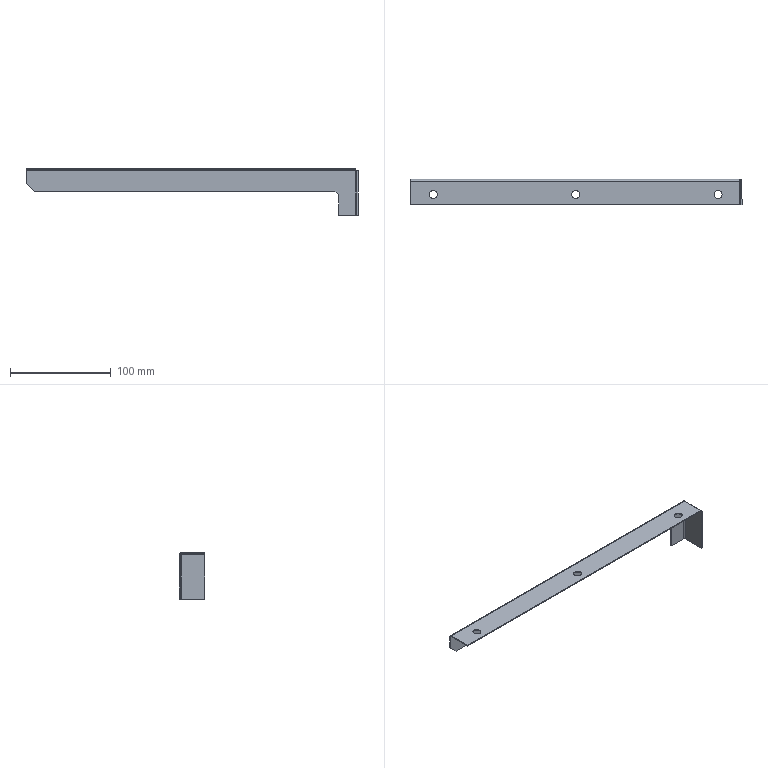Part | SolidWorks | features ICE 4, EdgeFlange 2, Chamfer 1, Fillet 1, FlatPattern 1, SMBaseFlange 1, SheetMetal 1 | 1 solid | 32 faces | box 330 x 25 x 46.5 mm | volume 16555 mm3 | plane 21 | cylinder 11 | commonest cylinder face diameters 8 x6 2 x2 4 x2 10 x1
STEP:
#1=CARTESIAN_POINT('',(-159.3,-14.,46.5));
#2=VERTEX_POINT('',#1);
#3=CARTESIAN_POINT('',(-167.3,-14.,46.5));
#4=VERTEX_POINT('',#3);
#5=CARTESIAN_POINT('',(-163.3,-14.,46.5));
#6=DIRECTION('',(0.,0.,-1.));
#7=DIRECTION('',(-1.,0.,0.));
#8=AXIS2_PLACEMENT_3D('',#5,#6,#7);
#9=CIRCLE('',#8,4.);
#10=EDGE_CURVE('',#2,#4,#9,.T.);
#11=ORIENTED_EDGE('',*,*,#10,.F.);
#12=CARTESIAN_POINT('',(-159.3,-14.,45.5));
#13=VERTEX_POINT('',#12);
#14=CARTESIAN_POINT('',(-159.3,-14.,46.5));
#15=DIRECTION('',(0.,0.,-1.));
#16=VECTOR('',#15,1000.);
#17=LINE('',#14,#16);
#18=EDGE_CURVE('',#2,#13,#17,.T.);
#19=ORIENTED_EDGE('',*,*,#18,.T.);
#20=CARTESIAN_POINT('',(-167.3,-14.,45.5));
#21=VERTEX_POINT('',#20);
#22=CARTESIAN_POINT('',(-163.3,-14.,45.5));
#23=DIRECTION('',(0.,0.,-1.));
#24=DIRECTION('',(-1.,0.,0.));
#25=AXIS2_PLACEMENT_3D('',#22,#23,#24);
#26=CIRCLE('',#25,4.);
#27=EDGE_CURVE('',#13,#21,#26,.T.);
#28=ORIENTED_EDGE('',*,*,#27,.T.);
#29=CARTESIAN_POINT('',(-167.3,-14.,46.5));
#30=DIRECTION('',(0.,0.,-1.));
#31=VECTOR('',#30,1000.);
#32=LINE('',#29,#31);
#33=EDGE_CURVE('',#4,#21,#32,.T.);
#34=ORIENTED_EDGE('',*,*,#33,.F.);
#35=EDGE_LOOP('',(#11,#19,#28,#34));
#36=FACE_OUTER_BOUND('',#35,.T.);
#37=CARTESIAN_POINT('',(-163.3,-14.,46.5));
#38=DIRECTION('',(0.,0.,-1.));
#39=DIRECTION('',(-1.,0.,0.));
#40=AXIS2_PLACEMENT_3D('',#37,#38,#39);
#41=CYLINDRICAL_SURFACE('',#40,4.);
#42=ADVANCED_FACE('',(#36),#41,.F.);
#43=CARTESIAN_POINT('',(-300.8,-14.,45.5));
#44=VERTEX_POINT('',#43);
#45=CARTESIAN_POINT('',(-308.8,-14.,45.5));
#46=VERTEX_POINT('',#45);
#47=CARTESIAN_POINT('',(-304.8,-14.,45.5));
#48=DIRECTION('',(0.,0.,-1.));
#49=DIRECTION('',(0.,-1.,0.));
#50=AXIS2_PLACEMENT_3D('',#47,#48,#49);
#51=CIRCLE('',#50,4.);
#52=EDGE_CURVE('',#44,#46,#51,.T.);
#53=ORIENTED_EDGE('',*,*,#52,.T.);
#54=CARTESIAN_POINT('',(-308.8,-14.,46.5));
#55=VERTEX_POINT('',#54);
#56=CARTESIAN_POINT('',(-308.8,-14.,-0.001));
#57=DIRECTION('',(0.,0.,1.));
#58=VECTOR('',#57,1000.);
#59=LINE('',#56,#58);
#60=EDGE_CURVE('',#46,#55,#59,.T.);
#61=ORIENTED_EDGE('',*,*,#60,.T.);
#62=CARTESIAN_POINT('',(-300.8,-14.,46.5));
#63=VERTEX_POINT('',#62);
#64=CARTESIAN_POINT('',(-304.8,-14.,46.5));
#65=DIRECTION('',(0.,0.,1.));
#66=DIRECTION('',(1.,0.,0.));
#67=AXIS2_PLACEMENT_3D('',#64,#65,#66);
#68=CIRCLE('',#67,4.);
#69=EDGE_CURVE('',#55,#63,#68,.T.);
#70=ORIENTED_EDGE('',*,*,#69,.T.);
#71=CARTESIAN_POINT('',(-300.8,-14.,-0.001));
#72=DIRECTION('',(0.,0.,1.));
#73=VECTOR('',#72,1000.);
#74=LINE('',#71,#73);
#75=EDGE_CURVE('',#44,#63,#74,.T.);
#76=ORIENTED_EDGE('',*,*,#75,.F.);
#77=EDGE_LOOP('',(#53,#61,#70,#76));
#78=FACE_OUTER_BOUND('',#77,.T.);
#79=CARTESIAN_POINT('',(-304.8,-14.,-0.001));
#80=DIRECTION('',(0.,0.,1.));
#81=DIRECTION('',(1.,0.,0.));
#82=AXIS2_PLACEMENT_3D('',#79,#80,#81);
#83=CYLINDRICAL_SURFACE('',#82,4.);
#84=ADVANCED_FACE('',(#78),#83,.F.);
#85=CARTESIAN_POINT('',(-17.8,-14.,45.5));
#86=VERTEX_POINT('',#85);
#87=CARTESIAN_POINT('',(-25.8,-14.,45.5));
#88=VERTEX_POINT('',#87);
#89=CARTESIAN_POINT('',(-21.8,-14.,45.5));
#90=DIRECTION('',(0.,0.,-1.));
#91=DIRECTION('',(0.,-1.,0.));
#92=AXIS2_PLACEMENT_3D('',#89,#90,#91);
#93=CIRCLE('',#92,4.);
#94=EDGE_CURVE('',#86,#88,#93,.T.);
#95=ORIENTED_EDGE('',*,*,#94,.T.);
#96=CARTESIAN_POINT('',(-25.8,-14.,46.5));
#97=VERTEX_POINT('',#96);
#98=CARTESIAN_POINT('',(-25.8,-14.,-0.001));
#99=DIRECTION('',(0.,0.,1.));
#100=VECTOR('',#99,1000.);
#101=LINE('',#98,#100);
#102=EDGE_CURVE('',#88,#97,#101,.T.);
#103=ORIENTED_EDGE('',*,*,#102,.T.);
#104=CARTESIAN_POINT('',(-17.8,-14.,46.5));
#105=VERTEX_POINT('',#104);
#106=CARTESIAN_POINT('',(-21.8,-14.,46.5));
#107=DIRECTION('',(0.,0.,1.));
#108=DIRECTION('',(1.,0.,0.));
#109=AXIS2_PLACEMENT_3D('',#106,#107,#108);
#110=CIRCLE('',#109,4.);
#111=EDGE_CURVE('',#97,#105,#110,.T.);
#112=ORIENTED_EDGE('',*,*,#111,.T.);
#113=CARTESIAN_POINT('',(-17.8,-14.,-0.001));
#114=DIRECTION('',(0.,0.,1.));
#115=VECTOR('',#114,1000.);
#116=LINE('',#113,#115);
#117=EDGE_CURVE('',#86,#105,#116,.T.);
#118=ORIENTED_EDGE('',*,*,#117,.F.);
#119=EDGE_LOOP('',(#95,#103,#112,#118));
#120=FACE_OUTER_BOUND('',#119,.T.);
#121=CARTESIAN_POINT('',(-21.8,-14.,-0.001));
#122=DIRECTION('',(0.,0.,1.));
#123=DIRECTION('',(1.,0.,0.));
#124=AXIS2_PLACEMENT_3D('',#121,#122,#123);
#125=CYLINDRICAL_SURFACE('',#124,4.);
#126=ADVANCED_FACE('',(#120),#125,.F.);
#127=CARTESIAN_POINT('',(-328.,0.,44.5));
#128=VERTEX_POINT('',#127);
#129=CARTESIAN_POINT('',(-328.,0.,31.5));
#130=VERTEX_POINT('',#129);
#131=CARTESIAN_POINT('',(-328.,0.,44.5));
#132=DIRECTION('',(0.,0.,-1.));
#133=VECTOR('',#132,1000.);
#134=LINE('',#131,#133);
#135=EDGE_CURVE('',#128,#130,#134,.T.);
#136=ORIENTED_EDGE('',*,*,#135,.T.);
#137=CARTESIAN_POINT('',(-320.,0.,23.5));
#138=VERTEX_POINT('',#137);
#139=CARTESIAN_POINT('',(-328.,0.,31.5));
#140=DIRECTION('',(0.7071,0.,-0.7071));
#141=VECTOR('',#140,1000.);
#142=LINE('',#139,#141);
#143=EDGE_CURVE('',#130,#138,#142,.T.);
#144=ORIENTED_EDGE('',*,*,#143,.T.);
#145=CARTESIAN_POINT('',(-22.,0.,23.5));
#146=VERTEX_POINT('',#145);
#147=CARTESIAN_POINT('',(-328.,0.,23.5));
#148=DIRECTION('',(-1.,0.,0.));
#149=VECTOR('',#148,1000.);
#150=LINE('',#147,#149);
#151=EDGE_CURVE('',#146,#138,#150,.T.);
#152=ORIENTED_EDGE('',*,*,#151,.F.);
#153=CARTESIAN_POINT('',(-17.,0.,18.5));
#154=VERTEX_POINT('',#153);
#155=CARTESIAN_POINT('',(-22.,0.,18.5));
#156=DIRECTION('',(0.,1.,0.));
#157=DIRECTION('',(0.,0.,1.));
#158=AXIS2_PLACEMENT_3D('',#155,#156,#157);
#159=CIRCLE('',#158,5.);
#160=EDGE_CURVE('',#146,#154,#159,.T.);
#161=ORIENTED_EDGE('',*,*,#160,.T.);
#162=CARTESIAN_POINT('',(-17.,0.,0.));
#163=VERTEX_POINT('',#162);
#164=CARTESIAN_POINT('',(-17.,0.,0.));
#165=DIRECTION('',(0.,0.,1.));
#166=VECTOR('',#165,1000.);
#167=LINE('',#164,#166);
#168=EDGE_CURVE('',#163,#154,#167,.T.);
#169=ORIENTED_EDGE('',*,*,#168,.F.);
#170=CARTESIAN_POINT('',(0.,0.,0.));
#171=VERTEX_POINT('',#170);
#172=CARTESIAN_POINT('',(-328.,0.,0.));
#173=DIRECTION('',(1.,0.,0.));
#174=VECTOR('',#173,1000.);
#175=LINE('',#172,#174);
#176=EDGE_CURVE('',#163,#171,#175,.T.);
#177=ORIENTED_EDGE('',*,*,#176,.T.);
#178=CARTESIAN_POINT('',(0.,0.,44.5));
#179=VERTEX_POINT('',#178);
#180=CARTESIAN_POINT('',(0.,0.,44.5));
#181=DIRECTION('',(0.,0.,-1.));
#182=VECTOR('',#181,1000.);
#183=LINE('',#180,#182);
#184=EDGE_CURVE('',#179,#171,#183,.T.);
#185=ORIENTED_EDGE('',*,*,#184,.F.);
#186=CARTESIAN_POINT('',(-328.,0.,44.5));
#187=DIRECTION('',(1.,0.,0.));
#188=VECTOR('',#187,1000.);
#189=LINE('',#186,#188);
#190=EDGE_CURVE('',#128,#179,#189,.T.);
#191=ORIENTED_EDGE('',*,*,#190,.F.);
#192=EDGE_LOOP('',(#136,#144,#152,#161,#169,#177,#185,#191));
#193=FACE_OUTER_BOUND('',#192,.T.);
#194=CARTESIAN_POINT('',(-328.,0.,44.5));
#195=DIRECTION('',(0.,1.,0.));
#196=DIRECTION('',(0.,0.,1.));
#197=AXIS2_PLACEMENT_3D('',#194,#195,#196);
#198=PLANE('',#197);
#199=ADVANCED_FACE('',(#193),#198,.F.);
#200=CARTESIAN_POINT('',(-320.,1.,23.5));
#201=VERTEX_POINT('',#200);
#202=CARTESIAN_POINT('',(-22.,1.,23.5));
#203=VERTEX_POINT('',#202);
#204=CARTESIAN_POINT('',(-328.,1.,23.5));
#205=DIRECTION('',(1.,0.,0.));
#206=VECTOR('',#205,1000.);
#207=LINE('',#204,#206);
#208=EDGE_CURVE('',#201,#203,#207,.T.);
#209=ORIENTED_EDGE('',*,*,#208,.F.);
#210=CARTESIAN_POINT('',(-328.,1.,31.5));
#211=VERTEX_POINT('',#210);
#212=CARTESIAN_POINT('',(-334.5,1.,38.));
#213=DIRECTION('',(-0.7071,0.,0.7071));
#214=VECTOR('',#213,1000.);
#215=LINE('',#212,#214);
#216=EDGE_CURVE('',#201,#211,#215,.T.);
#217=ORIENTED_EDGE('',*,*,#216,.T.);
#218=CARTESIAN_POINT('',(-328.,1.,44.5));
#219=VERTEX_POINT('',#218);
#220=CARTESIAN_POINT('',(-328.,1.,44.5));
#221=DIRECTION('',(0.,0.,-1.));
#222=VECTOR('',#221,1000.);
#223=LINE('',#220,#222);
#224=EDGE_CURVE('',#219,#211,#223,.T.);
#225=ORIENTED_EDGE('',*,*,#224,.F.);
#226=CARTESIAN_POINT('',(0.,1.,44.5));
#227=VERTEX_POINT('',#226);
#228=CARTESIAN_POINT('',(-328.,1.,44.5));
#229=DIRECTION('',(1.,0.,0.));
#230=VECTOR('',#229,1000.);
#231=LINE('',#228,#230);
#232=EDGE_CURVE('',#219,#227,#231,.T.);
#233=ORIENTED_EDGE('',*,*,#232,.T.);
#234=CARTESIAN_POINT('',(0.,1.,0.));
#235=VERTEX_POINT('',#234);
#236=CARTESIAN_POINT('',(0.,1.,44.5));
#237=DIRECTION('',(0.,0.,-1.));
#238=VECTOR('',#237,1000.);
#239=LINE('',#236,#238);
#240=EDGE_CURVE('',#227,#235,#239,.T.);
#241=ORIENTED_EDGE('',*,*,#240,.T.);
#242=CARTESIAN_POINT('',(-17.,1.,0.));
#243=VERTEX_POINT('',#242);
#244=CARTESIAN_POINT('',(-328.,1.,0.));
#245=DIRECTION('',(1.,0.,0.));
#246=VECTOR('',#245,1000.);
#247=LINE('',#244,#246);
#248=EDGE_CURVE('',#243,#235,#247,.T.);
#249=ORIENTED_EDGE('',*,*,#248,.F.);
#250=CARTESIAN_POINT('',(-17.,1.,18.5));
#251=VERTEX_POINT('',#250);
#252=CARTESIAN_POINT('',(-17.,1.,44.5));
#253=DIRECTION('',(0.,0.,-1.));
#254=VECTOR('',#253,1000.);
#255=LINE('',#252,#254);
#256=EDGE_CURVE('',#251,#243,#255,.T.);
#257=ORIENTED_EDGE('',*,*,#256,.F.);
#258=CARTESIAN_POINT('',(-22.,1.,18.5));
#259=DIRECTION('',(0.,-1.,0.));
#260=DIRECTION('',(0.,0.,1.));
#261=AXIS2_PLACEMENT_3D('',#258,#259,#260);
#262=CIRCLE('',#261,5.);
#263=EDGE_CURVE('',#251,#203,#262,.T.);
#264=ORIENTED_EDGE('',*,*,#263,.T.);
#265=EDGE_LOOP('',(#209,#217,#225,#233,#241,#249,#257,#264));
#266=FACE_OUTER_BOUND('',#265,.T.);
#267=CARTESIAN_POINT('',(-328.,1.,44.5));
#268=DIRECTION('',(0.,1.,0.));
#269=DIRECTION('',(0.,0.,1.));
#270=AXIS2_PLACEMENT_3D('',#267,#268,#269);
#271=PLANE('',#270);
#272=ADVANCED_FACE('',(#266),#271,.T.);
#273=ORIENTED_EDGE('',*,*,#224,.T.);
#274=CARTESIAN_POINT('',(-328.,0.,31.5));
#275=DIRECTION('',(0.,-1.,0.));
#276=VECTOR('',#275,1000.);
#277=LINE('',#274,#276);
#278=EDGE_CURVE('',#211,#130,#277,.T.);
#279=ORIENTED_EDGE('',*,*,#278,.T.);
#280=ORIENTED_EDGE('',*,*,#135,.F.);
#281=CARTESIAN_POINT('',(-328.,0.,44.5));
#282=DIRECTION('',(0.,1.,0.));
#283=VECTOR('',#282,1000.);
#284=LINE('',#281,#283);
#285=EDGE_CURVE('',#128,#219,#284,.T.);
#286=ORIENTED_EDGE('',*,*,#285,.T.);
#287=EDGE_LOOP('',(#273,#279,#280,#286));
#288=FACE_OUTER_BOUND('',#287,.T.);
#289=CARTESIAN_POINT('',(-328.,0.,44.5));
#290=DIRECTION('',(-1.,0.,0.));
#291=DIRECTION('',(0.,0.,1.));
#292=AXIS2_PLACEMENT_3D('',#289,#290,#291);
#293=PLANE('',#292);
#294=ADVANCED_FACE('',(#288),#293,.T.);
#295=CARTESIAN_POINT('',(-17.,0.,0.));
#296=DIRECTION('',(0.,-1.,0.));
#297=VECTOR('',#296,1000.);
#298=LINE('',#295,#297);
#299=EDGE_CURVE('',#243,#163,#298,.T.);
#300=ORIENTED_EDGE('',*,*,#299,.F.);
#301=ORIENTED_EDGE('',*,*,#248,.T.);
#302=CARTESIAN_POINT('',(0.,1.,0.));
#303=DIRECTION('',(0.,-1.,0.));
#304=VECTOR('',#303,1000.);
#305=LINE('',#302,#304);
#306=EDGE_CURVE('',#235,#171,#305,.T.);
#307=ORIENTED_EDGE('',*,*,#306,.T.);
#308=ORIENTED_EDGE('',*,*,#176,.F.);
#309=EDGE_LOOP('',(#300,#301,#307,#308));
#310=FACE_OUTER_BOUND('',#309,.T.);
#311=CARTESIAN_POINT('',(0.,0.,0.));
#312=DIRECTION('',(0.,0.,-1.));
#313=DIRECTION('',(-1.,0.,0.));
#314=AXIS2_PLACEMENT_3D('',#311,#312,#313);
#315=PLANE('',#314);
#316=ADVANCED_FACE('',(#310),#315,.T.);
#317=CARTESIAN_POINT('',(0.,-1.,45.5));
#318=VERTEX_POINT('',#317);
#319=CARTESIAN_POINT('',(0.,-1.,46.5));
#320=VERTEX_POINT('',#319);
#321=CARTESIAN_POINT('',(0.,-1.,46.5));
#322=DIRECTION('',(0.,0.,1.));
#323=VECTOR('',#322,1000.);
#324=LINE('',#321,#323);
#325=EDGE_CURVE('',#318,#320,#324,.T.);
#326=ORIENTED_EDGE('',*,*,#325,.F.);
#327=CARTESIAN_POINT('',(0.,-1.,44.5));
#328=DIRECTION('',(1.,0.,0.));
#329=DIRECTION('',(0.,0.,1.));
#330=AXIS2_PLACEMENT_3D('',#327,#328,#329);
#331=CIRCLE('',#330,1.);
#332=EDGE_CURVE('',#179,#318,#331,.T.);
#333=ORIENTED_EDGE('',*,*,#332,.F.);
#334=CARTESIAN_POINT('',(0.,1.,44.5));
#335=DIRECTION('',(0.,-1.,0.));
#336=VECTOR('',#335,1000.);
#337=LINE('',#334,#336);
#338=EDGE_CURVE('',#227,#179,#337,.T.);
#339=ORIENTED_EDGE('',*,*,#338,.F.);
#340=CARTESIAN_POINT('',(0.,-1.,44.5));
#341=DIRECTION('',(1.,0.,0.));
#342=DIRECTION('',(0.,0.,1.));
#343=AXIS2_PLACEMENT_3D('',#340,#341,#342);
#344=CIRCLE('',#343,2.);
#345=EDGE_CURVE('',#227,#320,#344,.T.);
#346=ORIENTED_EDGE('',*,*,#345,.T.);
#347=EDGE_LOOP('',(#326,#333,#339,#346));
#348=FACE_OUTER_BOUND('',#347,.T.);
#349=CARTESIAN_POINT('',(0.,-1.,44.5));
#350=DIRECTION('',(1.,0.,0.));
#351=DIRECTION('',(0.,0.,-1.));
#352=AXIS2_PLACEMENT_3D('',#349,#350,#351);
#353=PLANE('',#352);
#354=ADVANCED_FACE('',(#348),#353,.T.);
#355=CARTESIAN_POINT('',(-328.,-1.,45.5));
#356=VERTEX_POINT('',#355);
#357=CARTESIAN_POINT('',(-328.,-1.,44.5));
#358=DIRECTION('',(-1.,0.,0.));
#359=DIRECTION('',(0.,0.,1.));
#360=AXIS2_PLACEMENT_3D('',#357,#358,#359);
#361=CIRCLE('',#360,1.);
#362=EDGE_CURVE('',#356,#128,#361,.T.);
#363=ORIENTED_EDGE('',*,*,#362,.F.);
#364=CARTESIAN_POINT('',(-328.,-1.,46.5));
#365=VERTEX_POINT('',#364);
#366=CARTESIAN_POINT('',(-328.,-1.,45.5));
#367=DIRECTION('',(0.,0.,1.));
#368=VECTOR('',#367,1000.);
#369=LINE('',#366,#368);
#370=EDGE_CURVE('',#356,#365,#369,.T.);
#371=ORIENTED_EDGE('',*,*,#370,.T.);
#372=CARTESIAN_POINT('',(-328.,-1.,44.5));
#373=DIRECTION('',(-1.,0.,0.));
#374=DIRECTION('',(0.,0.,1.));
#375=AXIS2_PLACEMENT_3D('',#372,#373,#374);
#376=CIRCLE('',#375,2.);
#377=EDGE_CURVE('',#365,#219,#376,.T.);
#378=ORIENTED_EDGE('',*,*,#377,.T.);
#379=ORIENTED_EDGE('',*,*,#285,.F.);
#380=EDGE_LOOP('',(#363,#371,#378,#379));
#381=FACE_OUTER_BOUND('',#380,.T.);
#382=CARTESIAN_POINT('',(-328.,-1.,44.5));
#383=DIRECTION('',(1.,0.,0.));
#384=DIRECTION('',(0.,0.,-1.));
#385=AXIS2_PLACEMENT_3D('',#382,#383,#384);
#386=PLANE('',#385);
#387=ADVANCED_FACE('',(#381),#386,.F.);
#388=ORIENTED_EDGE('',*,*,#232,.F.);
#389=ORIENTED_EDGE('',*,*,#377,.F.);
#390=CARTESIAN_POINT('',(0.,-1.,46.5));
#391=DIRECTION('',(-1.,0.,0.));
#392=VECTOR('',#391,1000.);
#393=LINE('',#390,#392);
#394=EDGE_CURVE('',#320,#365,#393,.T.);
#395=ORIENTED_EDGE('',*,*,#394,.F.);
#396=ORIENTED_EDGE('',*,*,#345,.F.);
#397=EDGE_LOOP('',(#388,#389,#395,#396));
#398=FACE_OUTER_BOUND('',#397,.T.);
#399=CARTESIAN_POINT('',(-328.,-1.,44.5));
#400=DIRECTION('',(-1.,0.,0.));
#401=DIRECTION('',(0.,0.,1.));
#402=AXIS2_PLACEMENT_3D('',#399,#400,#401);
#403=CYLINDRICAL_SURFACE('',#402,2.);
#404=ADVANCED_FACE('',(#398),#403,.T.);
#405=ORIENTED_EDGE('',*,*,#190,.T.);
#406=ORIENTED_EDGE('',*,*,#332,.T.);
#407=CARTESIAN_POINT('',(0.,-1.,45.5));
#408=DIRECTION('',(-1.,0.,0.));
#409=VECTOR('',#408,1000.);
#410=LINE('',#407,#409);
#411=EDGE_CURVE('',#318,#356,#410,.T.);
#412=ORIENTED_EDGE('',*,*,#411,.T.);
#413=ORIENTED_EDGE('',*,*,#362,.T.);
#414=EDGE_LOOP('',(#405,#406,#412,#413));
#415=FACE_OUTER_BOUND('',#414,.T.);
#416=CARTESIAN_POINT('',(-328.,-1.,44.5));
#417=DIRECTION('',(-1.,0.,0.));
#418=DIRECTION('',(0.,0.,1.));
#419=AXIS2_PLACEMENT_3D('',#416,#417,#418);
#420=CYLINDRICAL_SURFACE('',#419,1.);
#421=ADVANCED_FACE('',(#415),#420,.F.);
#422=CARTESIAN_POINT('',(-328.,-24.,46.5));
#423=VERTEX_POINT('',#422);
#424=CARTESIAN_POINT('',(-328.,0.,46.5));
#425=DIRECTION('',(0.,1.,0.));
#426=VECTOR('',#425,1000.);
#427=LINE('',#424,#426);
#428=EDGE_CURVE('',#423,#365,#427,.T.);
#429=ORIENTED_EDGE('',*,*,#428,.T.);
#430=ORIENTED_EDGE('',*,*,#370,.F.);
#431=CARTESIAN_POINT('',(-328.,-24.,45.5));
#432=VERTEX_POINT('',#431);
#433=CARTESIAN_POINT('',(-328.,0.,45.5));
#434=DIRECTION('',(0.,1.,0.));
#435=VECTOR('',#434,1000.);
#436=LINE('',#433,#435);
#437=EDGE_CURVE('',#432,#356,#436,.T.);
#438=ORIENTED_EDGE('',*,*,#437,.F.);
#439=CARTESIAN_POINT('',(-328.,-24.,46.5));
#440=DIRECTION('',(0.,0.,-1.));
#441=VECTOR('',#440,1000.);
#442=LINE('',#439,#441);
#443=EDGE_CURVE('',#423,#432,#442,.T.);
#444=ORIENTED_EDGE('',*,*,#443,.F.);
#445=EDGE_LOOP('',(#429,#430,#438,#444));
#446=FACE_OUTER_BOUND('',#445,.T.);
#447=CARTESIAN_POINT('',(-328.,0.,46.5));
#448=DIRECTION('',(-1.,0.,0.));
#449=DIRECTION('',(0.,0.,1.));
#450=AXIS2_PLACEMENT_3D('',#447,#448,#449);
#451=PLANE('',#450);
#452=ADVANCED_FACE('',(#446),#451,.T.);
#453=CARTESIAN_POINT('',(0.,-24.,45.5));
#454=VERTEX_POINT('',#453);
#455=CARTESIAN_POINT('',(0.,0.,45.5));
#456=DIRECTION('',(0.,-1.,0.));
#457=VECTOR('',#456,1000.);
#458=LINE('',#455,#457);
#459=EDGE_CURVE('',#318,#454,#458,.T.);
#460=ORIENTED_EDGE('',*,*,#459,.F.);
#461=ORIENTED_EDGE('',*,*,#325,.T.);
#462=CARTESIAN_POINT('',(0.,-24.,46.5));
#463=VERTEX_POINT('',#462);
#464=CARTESIAN_POINT('',(0.,-24.,46.5));
#465=DIRECTION('',(0.,-1.,0.));
#466=VECTOR('',#465,1000.);
#467=LINE('',#464,#466);
#468=EDGE_CURVE('',#320,#463,#467,.T.);
#469=ORIENTED_EDGE('',*,*,#468,.T.);
#470=CARTESIAN_POINT('',(0.,-24.,46.5));
#471=DIRECTION('',(0.,0.,-1.));
#472=VECTOR('',#471,1000.);
#473=LINE('',#470,#472);
#474=EDGE_CURVE('',#463,#454,#473,.T.);
#475=ORIENTED_EDGE('',*,*,#474,.T.);
#476=EDGE_LOOP('',(#460,#461,#469,#475));
#477=FACE_OUTER_BOUND('',#476,.T.);
#478=CARTESIAN_POINT('',(0.,-24.,46.5));
#479=DIRECTION('',(1.,0.,0.));
#480=DIRECTION('',(0.,0.,-1.));
#481=AXIS2_PLACEMENT_3D('',#478,#479,#480);
#482=PLANE('',#481);
#483=ADVANCED_FACE('',(#477),#482,.T.);
#484=CARTESIAN_POINT('',(-163.3,-14.,46.5));
#485=DIRECTION('',(0.,0.,-1.));
#486=DIRECTION('',(-1.,0.,0.));
#487=AXIS2_PLACEMENT_3D('',#484,#485,#486);
#488=CIRCLE('',#487,4.);
#489=EDGE_CURVE('',#4,#2,#488,.T.);
#490=ORIENTED_EDGE('',*,*,#489,.T.);
#491=ORIENTED_EDGE('',*,*,#10,.T.);
#492=EDGE_LOOP('',(#490,#491));
#493=FACE_BOUND('',#492,.T.);
#494=CARTESIAN_POINT('',(-304.8,-14.,46.5));
#495=DIRECTION('',(0.,0.,1.));
#496=DIRECTION('',(1.,0.,0.));
#497=AXIS2_PLACEMENT_3D('',#494,#495,#496);
#498=CIRCLE('',#497,4.);
#499=EDGE_CURVE('',#63,#55,#498,.T.);
#500=ORIENTED_EDGE('',*,*,#499,.F.);
#501=ORIENTED_EDGE('',*,*,#69,.F.);
#502=EDGE_LOOP('',(#500,#501));
#503=FACE_BOUND('',#502,.T.);
#504=CARTESIAN_POINT('',(-21.8,-14.,46.5));
#505=DIRECTION('',(0.,0.,1.));
#506=DIRECTION('',(1.,0.,0.));
#507=AXIS2_PLACEMENT_3D('',#504,#505,#506);
#508=CIRCLE('',#507,4.);
#509=EDGE_CURVE('',#105,#97,#508,.T.);
#510=ORIENTED_EDGE('',*,*,#509,.F.);
#511=ORIENTED_EDGE('',*,*,#111,.F.);
#512=EDGE_LOOP('',(#510,#511));
#513=FACE_BOUND('',#512,.T.);
#514=ORIENTED_EDGE('',*,*,#468,.F.);
#515=ORIENTED_EDGE('',*,*,#394,.T.);
#516=ORIENTED_EDGE('',*,*,#428,.F.);
#517=CARTESIAN_POINT('',(-328.,-24.,46.5));
#518=DIRECTION('',(-1.,0.,0.));
#519=VECTOR('',#518,1000.);
#520=LINE('',#517,#519);
#521=EDGE_CURVE('',#463,#423,#520,.T.);
#522=ORIENTED_EDGE('',*,*,#521,.F.);
#523=EDGE_LOOP('',(#514,#515,#516,#522));
#524=FACE_OUTER_BOUND('',#523,.T.);
#525=CARTESIAN_POINT('',(0.,0.,46.5));
#526=DIRECTION('',(0.,0.,1.));
#527=DIRECTION('',(0.,-1.,0.));
#528=AXIS2_PLACEMENT_3D('',#525,#526,#527);
#529=PLANE('',#528);
#530=ADVANCED_FACE('',(#493,#503,#513,#524),#529,.T.);
#531=CARTESIAN_POINT('',(-163.3,-14.,45.5));
#532=DIRECTION('',(0.,0.,-1.));
#533=DIRECTION('',(-1.,0.,0.));
#534=AXIS2_PLACEMENT_3D('',#531,#532,#533);
#535=CIRCLE('',#534,4.);
#536=EDGE_CURVE('',#21,#13,#535,.T.);
#537=ORIENTED_EDGE('',*,*,#536,.F.);
#538=ORIENTED_EDGE('',*,*,#27,.F.);
#539=EDGE_LOOP('',(#537,#538));
#540=FACE_BOUND('',#539,.T.);
#541=ORIENTED_EDGE('',*,*,#52,.F.);
#542=CARTESIAN_POINT('',(-304.8,-14.,45.5));
#543=DIRECTION('',(0.,0.,-1.));
#544=DIRECTION('',(0.,-1.,0.));
#545=AXIS2_PLACEMENT_3D('',#542,#543,#544);
#546=CIRCLE('',#545,4.);
#547=EDGE_CURVE('',#46,#44,#546,.T.);
#548=ORIENTED_EDGE('',*,*,#547,.F.);
#549=EDGE_LOOP('',(#541,#548));
#550=FACE_BOUND('',#549,.T.);
#551=ORIENTED_EDGE('',*,*,#94,.F.);
#552=CARTESIAN_POINT('',(-21.8,-14.,45.5));
#553=DIRECTION('',(0.,0.,-1.));
#554=DIRECTION('',(0.,-1.,0.));
#555=AXIS2_PLACEMENT_3D('',#552,#553,#554);
#556=CIRCLE('',#555,4.);
#557=EDGE_CURVE('',#88,#86,#556,.T.);
#558=ORIENTED_EDGE('',*,*,#557,.F.);
#559=EDGE_LOOP('',(#551,#558));
#560=FACE_BOUND('',#559,.T.);
#561=ORIENTED_EDGE('',*,*,#411,.F.);
#562=ORIENTED_EDGE('',*,*,#459,.T.);
#563=CARTESIAN_POINT('',(0.,-24.,45.5));
#564=DIRECTION('',(-1.,0.,0.));
#565=VECTOR('',#564,1000.);
#566=LINE('',#563,#565);
#567=EDGE_CURVE('',#454,#432,#566,.T.);
#568=ORIENTED_EDGE('',*,*,#567,.T.);
#569=ORIENTED_EDGE('',*,*,#437,.T.);
#570=EDGE_LOOP('',(#561,#562,#568,#569));
#571=FACE_OUTER_BOUND('',#570,.T.);
#572=CARTESIAN_POINT('',(0.,0.,45.5));
#573=DIRECTION('',(0.,0.,1.));
#574=DIRECTION('',(0.,-1.,0.));
#575=AXIS2_PLACEMENT_3D('',#572,#573,#574);
#576=PLANE('',#575);
#577=ADVANCED_FACE('',(#540,#550,#560,#571),#576,.F.);
#578=ORIENTED_EDGE('',*,*,#567,.F.);
#579=ORIENTED_EDGE('',*,*,#474,.F.);
#580=ORIENTED_EDGE('',*,*,#521,.T.);
#581=ORIENTED_EDGE('',*,*,#443,.T.);
#582=EDGE_LOOP('',(#578,#579,#580,#581));
#583=FACE_OUTER_BOUND('',#582,.T.);
#584=CARTESIAN_POINT('',(-328.,-24.,46.5));
#585=DIRECTION('',(0.,-1.,0.));
#586=DIRECTION('',(0.,0.,-1.));
#587=AXIS2_PLACEMENT_3D('',#584,#585,#586);
#588=PLANE('',#587);
#589=ADVANCED_FACE('',(#583),#588,.T.);
#590=CARTESIAN_POINT('',(1.,-1.,0.));
#591=VERTEX_POINT('',#590);
#592=CARTESIAN_POINT('',(2.,-1.,0.));
#593=VERTEX_POINT('',#592);
#594=CARTESIAN_POINT('',(2.,-1.,0.));
#595=DIRECTION('',(1.,0.,0.));
#596=VECTOR('',#595,1000.);
#597=LINE('',#594,#596);
#598=EDGE_CURVE('',#591,#593,#597,.T.);
#599=ORIENTED_EDGE('',*,*,#598,.F.);
#600=CARTESIAN_POINT('',(0.,-1.,0.));
#601=DIRECTION('',(0.,0.,-1.));
#602=DIRECTION('',(0.,-1.,0.));
#603=AXIS2_PLACEMENT_3D('',#600,#601,#602);
#604=CIRCLE('',#603,1.);
#605=EDGE_CURVE('',#171,#591,#604,.T.);
#606=ORIENTED_EDGE('',*,*,#605,.F.);
#607=ORIENTED_EDGE('',*,*,#306,.F.);
#608=CARTESIAN_POINT('',(0.,-1.,0.));
#609=DIRECTION('',(0.,0.,-1.));
#610=DIRECTION('',(0.,-1.,0.));
#611=AXIS2_PLACEMENT_3D('',#608,#609,#610);
#612=CIRCLE('',#611,2.);
#613=EDGE_CURVE('',#235,#593,#612,.T.);
#614=ORIENTED_EDGE('',*,*,#613,.T.);
#615=EDGE_LOOP('',(#599,#606,#607,#614));
#616=FACE_OUTER_BOUND('',#615,.T.);
#617=CARTESIAN_POINT('',(0.,-1.,0.));
#618=DIRECTION('',(0.,0.,-1.));
#619=DIRECTION('',(0.,1.,0.));
#620=AXIS2_PLACEMENT_3D('',#617,#618,#619);
#621=PLANE('',#620);
#622=ADVANCED_FACE('',(#616),#621,.T.);
#623=CARTESIAN_POINT('',(1.,-1.,44.5));
#624=VERTEX_POINT('',#623);
#625=CARTESIAN_POINT('',(0.,-1.,44.5));
#626=DIRECTION('',(0.,0.,1.));
#627=DIRECTION('',(0.,-1.,0.));
#628=AXIS2_PLACEMENT_3D('',#625,#626,#627);
#629=CIRCLE('',#628,1.);
#630=EDGE_CURVE('',#624,#179,#629,.T.);
#631=ORIENTED_EDGE('',*,*,#630,.F.);
#632=CARTESIAN_POINT('',(2.,-1.,44.5));
#633=VERTEX_POINT('',#632);
#634=CARTESIAN_POINT('',(1.,-1.,44.5));
#635=DIRECTION('',(1.,0.,0.));
#636=VECTOR('',#635,1000.);
#637=LINE('',#634,#636);
#638=EDGE_CURVE('',#624,#633,#637,.T.);
#639=ORIENTED_EDGE('',*,*,#638,.T.);
#640=CARTESIAN_POINT('',(0.,-1.,44.5));
#641=DIRECTION('',(0.,0.,1.));
#642=DIRECTION('',(0.,-1.,0.));
#643=AXIS2_PLACEMENT_3D('',#640,#641,#642);
#644=CIRCLE('',#643,2.);
#645=EDGE_CURVE('',#633,#227,#644,.T.);
#646=ORIENTED_EDGE('',*,*,#645,.T.);
#647=ORIENTED_EDGE('',*,*,#338,.T.);
#648=EDGE_LOOP('',(#631,#639,#646,#647));
#649=FACE_OUTER_BOUND('',#648,.T.);
#650=CARTESIAN_POINT('',(0.,-1.,44.5));
#651=DIRECTION('',(0.,0.,-1.));
#652=DIRECTION('',(0.,1.,0.));
#653=AXIS2_PLACEMENT_3D('',#650,#651,#652);
#654=PLANE('',#653);
#655=ADVANCED_FACE('',(#649),#654,.F.);
#656=ORIENTED_EDGE('',*,*,#240,.F.);
#657=ORIENTED_EDGE('',*,*,#645,.F.);
#658=CARTESIAN_POINT('',(2.,-1.,0.));
#659=DIRECTION('',(0.,0.,1.));
#660=VECTOR('',#659,1000.);
#661=LINE('',#658,#660);
#662=EDGE_CURVE('',#593,#633,#661,.T.);
#663=ORIENTED_EDGE('',*,*,#662,.F.);
#664=ORIENTED_EDGE('',*,*,#613,.F.);
#665=EDGE_LOOP('',(#656,#657,#663,#664));
#666=FACE_OUTER_BOUND('',#665,.T.);
#667=CARTESIAN_POINT('',(0.,-1.,44.5));
#668=DIRECTION('',(0.,0.,1.));
#669=DIRECTION('',(1.,0.,0.));
#670=AXIS2_PLACEMENT_3D('',#667,#668,#669);
#671=CYLINDRICAL_SURFACE('',#670,2.);
#672=ADVANCED_FACE('',(#666),#671,.T.);
#673=ORIENTED_EDGE('',*,*,#184,.T.);
#674=ORIENTED_EDGE('',*,*,#605,.T.);
#675=CARTESIAN_POINT('',(1.,-1.,0.));
#676=DIRECTION('',(0.,0.,1.));
#677=VECTOR('',#676,1000.);
#678=LINE('',#675,#677);
#679=EDGE_CURVE('',#591,#624,#678,.T.);
#680=ORIENTED_EDGE('',*,*,#679,.T.);
#681=ORIENTED_EDGE('',*,*,#630,.T.);
#682=EDGE_LOOP('',(#673,#674,#680,#681));
#683=FACE_OUTER_BOUND('',#682,.T.);
#684=CARTESIAN_POINT('',(0.,-1.,44.5));
#685=DIRECTION('',(0.,0.,1.));
#686=DIRECTION('',(1.,0.,0.));
#687=AXIS2_PLACEMENT_3D('',#684,#685,#686);
#688=CYLINDRICAL_SURFACE('',#687,1.);
#689=ADVANCED_FACE('',(#683),#688,.F.);
#690=CARTESIAN_POINT('',(2.,-24.,44.5));
#691=VERTEX_POINT('',#690);
#692=CARTESIAN_POINT('',(2.,0.,44.5));
#693=DIRECTION('',(0.,1.,0.));
#694=VECTOR('',#693,1000.);
#695=LINE('',#692,#694);
#696=EDGE_CURVE('',#691,#633,#695,.T.);
#697=ORIENTED_EDGE('',*,*,#696,.T.);
#698=ORIENTED_EDGE('',*,*,#638,.F.);
#699=CARTESIAN_POINT('',(1.,-24.,44.5));
#700=VERTEX_POINT('',#699);
#701=CARTESIAN_POINT('',(1.,0.,44.5));
#702=DIRECTION('',(0.,1.,0.));
#703=VECTOR('',#702,1000.);
#704=LINE('',#701,#703);
#705=EDGE_CURVE('',#700,#624,#704,.T.);
#706=ORIENTED_EDGE('',*,*,#705,.F.);
#707=CARTESIAN_POINT('',(2.,-24.,44.5));
#708=DIRECTION('',(-1.,0.,0.));
#709=VECTOR('',#708,1000.);
#710=LINE('',#707,#709);
#711=EDGE_CURVE('',#691,#700,#710,.T.);
#712=ORIENTED_EDGE('',*,*,#711,.F.);
#713=EDGE_LOOP('',(#697,#698,#706,#712));
#714=FACE_OUTER_BOUND('',#713,.T.);
#715=CARTESIAN_POINT('',(2.,0.,44.5));
#716=DIRECTION('',(0.,0.,1.));
#717=DIRECTION('',(0.,-1.,0.));
#718=AXIS2_PLACEMENT_3D('',#715,#716,#717);
#719=PLANE('',#718);
#720=ADVANCED_FACE('',(#714),#719,.T.);
#721=CARTESIAN_POINT('',(1.,-24.,0.));
#722=VERTEX_POINT('',#721);
#723=CARTESIAN_POINT('',(1.,0.,0.));
#724=DIRECTION('',(0.,-1.,0.));
#725=VECTOR('',#724,1000.);
#726=LINE('',#723,#725);
#727=EDGE_CURVE('',#591,#722,#726,.T.);
#728=ORIENTED_EDGE('',*,*,#727,.F.);
#729=ORIENTED_EDGE('',*,*,#598,.T.);
#730=CARTESIAN_POINT('',(2.,-24.,0.));
#731=VERTEX_POINT('',#730);
#732=CARTESIAN_POINT('',(2.,-24.,0.));
#733=DIRECTION('',(0.,-1.,0.));
#734=VECTOR('',#733,1000.);
#735=LINE('',#732,#734);
#736=EDGE_CURVE('',#593,#731,#735,.T.);
#737=ORIENTED_EDGE('',*,*,#736,.T.);
#738=CARTESIAN_POINT('',(2.,-24.,0.));
#739=DIRECTION('',(-1.,0.,0.));
#740=VECTOR('',#739,1000.);
#741=LINE('',#738,#740);
#742=EDGE_CURVE('',#731,#722,#741,.T.);
#743=ORIENTED_EDGE('',*,*,#742,.T.);
#744=EDGE_LOOP('',(#728,#729,#737,#743));
#745=FACE_OUTER_BOUND('',#744,.T.);
#746=CARTESIAN_POINT('',(2.,-24.,0.));
#747=DIRECTION('',(0.,0.,-1.));
#748=DIRECTION('',(0.,1.,0.));
#749=AXIS2_PLACEMENT_3D('',#746,#747,#748);
#750=PLANE('',#749);
#751=ADVANCED_FACE('',(#745),#750,.T.);
#752=ORIENTED_EDGE('',*,*,#736,.F.);
#753=ORIENTED_EDGE('',*,*,#662,.T.);
#754=ORIENTED_EDGE('',*,*,#696,.F.);
#755=CARTESIAN_POINT('',(2.,-24.,44.5));
#756=DIRECTION('',(0.,0.,1.));
#757=VECTOR('',#756,1000.);
#758=LINE('',#755,#757);
#759=EDGE_CURVE('',#731,#691,#758,.T.);
#760=ORIENTED_EDGE('',*,*,#759,.F.);
#761=EDGE_LOOP('',(#752,#753,#754,#760));
#762=FACE_OUTER_BOUND('',#761,.T.);
#763=CARTESIAN_POINT('',(2.,0.,0.));
#764=DIRECTION('',(1.,0.,0.));
#765=DIRECTION('',(0.,1.,0.));
#766=AXIS2_PLACEMENT_3D('',#763,#764,#765);
#767=PLANE('',#766);
#768=ADVANCED_FACE('',(#762),#767,.T.);
#769=ORIENTED_EDGE('',*,*,#679,.F.);
#770=ORIENTED_EDGE('',*,*,#727,.T.);
#771=CARTESIAN_POINT('',(1.,-24.,0.));
#772=DIRECTION('',(0.,0.,1.));
#773=VECTOR('',#772,1000.);
#774=LINE('',#771,#773);
#775=EDGE_CURVE('',#722,#700,#774,.T.);
#776=ORIENTED_EDGE('',*,*,#775,.T.);
#777=ORIENTED_EDGE('',*,*,#705,.T.);
#778=EDGE_LOOP('',(#769,#770,#776,#777));
#779=FACE_OUTER_BOUND('',#778,.T.);
#780=CARTESIAN_POINT('',(1.,0.,0.));
#781=DIRECTION('',(1.,0.,0.));
#782=DIRECTION('',(0.,1.,0.));
#783=AXIS2_PLACEMENT_3D('',#780,#781,#782);
#784=PLANE('',#783);
#785=ADVANCED_FACE('',(#779),#784,.F.);
#786=ORIENTED_EDGE('',*,*,#775,.F.);
#787=ORIENTED_EDGE('',*,*,#742,.F.);
#788=ORIENTED_EDGE('',*,*,#759,.T.);
#789=ORIENTED_EDGE('',*,*,#711,.T.);
#790=EDGE_LOOP('',(#786,#787,#788,#789));
#791=FACE_OUTER_BOUND('',#790,.T.);
#792=CARTESIAN_POINT('',(2.,-24.,44.5));
#793=DIRECTION('',(0.,-1.,0.));
#794=DIRECTION('',(1.,0.,0.));
#795=AXIS2_PLACEMENT_3D('',#792,#793,#794);
#796=PLANE('',#795);
#797=ADVANCED_FACE('',(#791),#796,.T.);
#798=ORIENTED_EDGE('',*,*,#151,.T.);
#799=CARTESIAN_POINT('',(-320.,1.,23.5));
#800=DIRECTION('',(0.,1.,0.));
#801=VECTOR('',#800,1000.);
#802=LINE('',#799,#801);
#803=EDGE_CURVE('',#138,#201,#802,.T.);
#804=ORIENTED_EDGE('',*,*,#803,.T.);
#805=ORIENTED_EDGE('',*,*,#208,.T.);
#806=CARTESIAN_POINT('',(-22.,0.,23.5));
#807=DIRECTION('',(0.,-1.,0.));
#808=VECTOR('',#807,1000.);
#809=LINE('',#806,#808);
#810=EDGE_CURVE('',#203,#146,#809,.T.);
#811=ORIENTED_EDGE('',*,*,#810,.T.);
#812=EDGE_LOOP('',(#798,#804,#805,#811));
#813=FACE_OUTER_BOUND('',#812,.T.);
#814=CARTESIAN_POINT('',(-328.,10.,23.5));
#815=DIRECTION('',(0.,0.,1.));
#816=DIRECTION('',(1.,0.,0.));
#817=AXIS2_PLACEMENT_3D('',#814,#815,#816);
#818=PLANE('',#817);
#819=ADVANCED_FACE('',(#813),#818,.F.);
#820=ORIENTED_EDGE('',*,*,#168,.T.);
#821=CARTESIAN_POINT('',(-17.,1.,18.5));
#822=DIRECTION('',(0.,1.,0.));
#823=VECTOR('',#822,1000.);
#824=LINE('',#821,#823);
#825=EDGE_CURVE('',#154,#251,#824,.T.);
#826=ORIENTED_EDGE('',*,*,#825,.T.);
#827=ORIENTED_EDGE('',*,*,#256,.T.);
#828=ORIENTED_EDGE('',*,*,#299,.T.);
#829=EDGE_LOOP('',(#820,#826,#827,#828));
#830=FACE_OUTER_BOUND('',#829,.T.);
#831=CARTESIAN_POINT('',(-17.,10.,0.));
#832=DIRECTION('',(1.,0.,0.));
#833=DIRECTION('',(0.,0.,-1.));
#834=AXIS2_PLACEMENT_3D('',#831,#832,#833);
#835=PLANE('',#834);
#836=ADVANCED_FACE('',(#830),#835,.F.);
#837=ORIENTED_EDGE('',*,*,#263,.F.);
#838=ORIENTED_EDGE('',*,*,#825,.F.);
#839=ORIENTED_EDGE('',*,*,#160,.F.);
#840=ORIENTED_EDGE('',*,*,#810,.F.);
#841=EDGE_LOOP('',(#837,#838,#839,#840));
#842=FACE_OUTER_BOUND('',#841,.T.);
#843=CARTESIAN_POINT('',(-22.,10.,18.5));
#844=DIRECTION('',(0.,1.,0.));
#845=DIRECTION('',(0.,0.,1.));
#846=AXIS2_PLACEMENT_3D('',#843,#844,#845);
#847=CYLINDRICAL_SURFACE('',#846,5.);
#848=ADVANCED_FACE('',(#842),#847,.F.);
#849=ORIENTED_EDGE('',*,*,#216,.F.);
#850=ORIENTED_EDGE('',*,*,#803,.F.);
#851=ORIENTED_EDGE('',*,*,#143,.F.);
#852=ORIENTED_EDGE('',*,*,#278,.F.);
#853=EDGE_LOOP('',(#849,#850,#851,#852));
#854=FACE_OUTER_BOUND('',#853,.T.);
#855=CARTESIAN_POINT('',(-328.,0.,31.5));
#856=DIRECTION('',(-0.7071,0.,-0.7071));
#857=DIRECTION('',(0.,1.,0.));
#858=AXIS2_PLACEMENT_3D('',#855,#856,#857);
#859=PLANE('',#858);
#860=ADVANCED_FACE('',(#854),#859,.T.);
#861=ORIENTED_EDGE('',*,*,#102,.F.);
#862=ORIENTED_EDGE('',*,*,#557,.T.);
#863=ORIENTED_EDGE('',*,*,#117,.T.);
#864=ORIENTED_EDGE('',*,*,#509,.T.);
#865=EDGE_LOOP('',(#861,#862,#863,#864));
#866=FACE_OUTER_BOUND('',#865,.T.);
#867=CARTESIAN_POINT('',(-21.8,-14.,-0.001));
#868=DIRECTION('',(0.,0.,1.));
#869=DIRECTION('',(1.,0.,0.));
#870=AXIS2_PLACEMENT_3D('',#867,#868,#869);
#871=CYLINDRICAL_SURFACE('',#870,4.);
#872=ADVANCED_FACE('',(#866),#871,.F.);
#873=ORIENTED_EDGE('',*,*,#60,.F.);
#874=ORIENTED_EDGE('',*,*,#547,.T.);
#875=ORIENTED_EDGE('',*,*,#75,.T.);
#876=ORIENTED_EDGE('',*,*,#499,.T.);
#877=EDGE_LOOP('',(#873,#874,#875,#876));
#878=FACE_OUTER_BOUND('',#877,.T.);
#879=CARTESIAN_POINT('',(-304.8,-14.,-0.001));
#880=DIRECTION('',(0.,0.,1.));
#881=DIRECTION('',(1.,0.,0.));
#882=AXIS2_PLACEMENT_3D('',#879,#880,#881);
#883=CYLINDRICAL_SURFACE('',#882,4.);
#884=ADVANCED_FACE('',(#878),#883,.F.);
#885=ORIENTED_EDGE('',*,*,#18,.F.);
#886=ORIENTED_EDGE('',*,*,#489,.F.);
#887=ORIENTED_EDGE('',*,*,#33,.T.);
#888=ORIENTED_EDGE('',*,*,#536,.T.);
#889=EDGE_LOOP('',(#885,#886,#887,#888));
#890=FACE_OUTER_BOUND('',#889,.T.);
#891=CARTESIAN_POINT('',(-163.3,-14.,46.5));
#892=DIRECTION('',(0.,0.,-1.));
#893=DIRECTION('',(-1.,0.,0.));
#894=AXIS2_PLACEMENT_3D('',#891,#892,#893);
#895=CYLINDRICAL_SURFACE('',#894,4.);
#896=ADVANCED_FACE('',(#890),#895,.F.);
#897=CLOSED_SHELL('',(#42,#84,#126,#199,#272,#294,#316,#354,#387,#404,#421,#452,#483,#530,#577,#589,#622,#655,#672,#689,#720,#751,#768,#785,#797,#819,#836,#848,#860,#872,#884,#896));
#898=MANIFOLD_SOLID_BREP('',#897);
#899=CARTESIAN_POINT('',(0.,0.,0.));
#900=DIRECTION('',(0.,0.,1.));
#901=DIRECTION('',(1.,0.,0.));
#902=AXIS2_PLACEMENT_3D('',#899,#900,#901);
#903=(LENGTH_UNIT()NAMED_UNIT(*)SI_UNIT(.MILLI.,.METRE.));
#904=UNCERTAINTY_MEASURE_WITH_UNIT(LENGTH_MEASURE(0.00001),#903,'','');
#905=(NAMED_UNIT(*)PLANE_ANGLE_UNIT()SI_UNIT($,.RADIAN.));
#906=(NAMED_UNIT(*)SI_UNIT($,.STERADIAN.)SOLID_ANGLE_UNIT());
#907=(GEOMETRIC_REPRESENTATION_CONTEXT(3)GLOBAL_UNCERTAINTY_ASSIGNED_CONTEXT((#904))GLOBAL_UNIT_ASSIGNED_CONTEXT((#903,#905,#906))REPRESENTATION_CONTEXT('',''));
#908=ADVANCED_BREP_SHAPE_REPRESENTATION('',(#898,#902),#907);